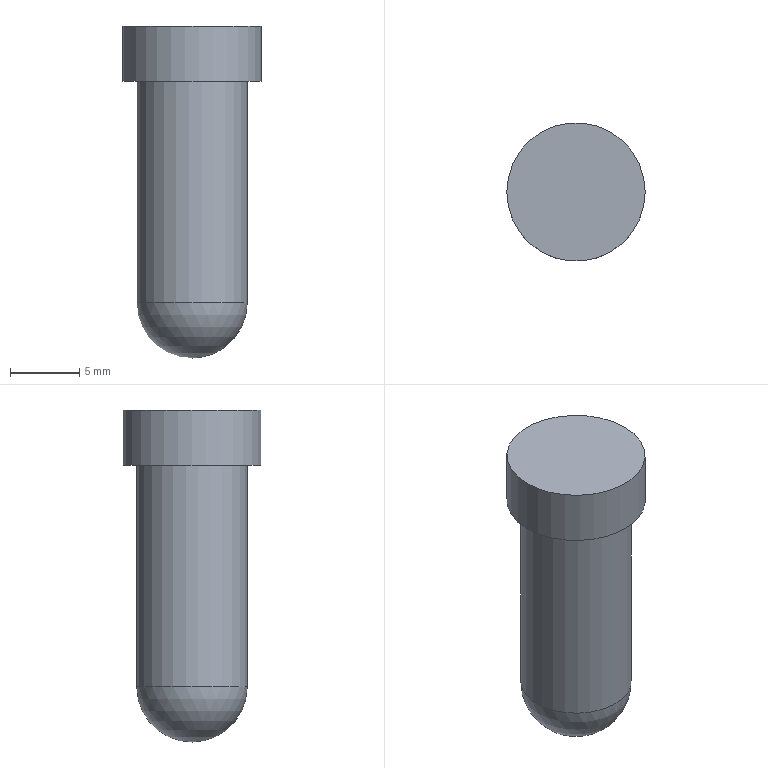Part | NX | features solid 2 | 1 solid | 5 faces | box 10 x 10 x 24 mm | volume 1252 mm3 | cylinder 2 | plane 2 | sphere 1 | commonest cylinder face diameters 8 x1 10 x1
STEP:
#1=CARTESIAN_POINT('',(-41.,110.,-78.));
#2=VERTEX_POINT('',#1);
#3=CARTESIAN_POINT('',(-45.,110.,-78.));
#4=DIRECTION('',(0.,0.,1.));
#5=DIRECTION('',(1.,0.,0.));
#6=AXIS2_PLACEMENT_3D('',#3,#4,#5);
#7=CIRCLE('',#6,4.);
#8=EDGE_CURVE('',#2,#2,#7,.F.);
#9=ORIENTED_EDGE('',*,*,#8,.F.);
#10=EDGE_LOOP('',(#9));
#11=FACE_BOUND('',#10,.T.);
#12=CARTESIAN_POINT('',(-41.,110.,-62.));
#13=VERTEX_POINT('',#12);
#14=CARTESIAN_POINT('',(-45.,110.,-62.));
#15=DIRECTION('',(0.,0.,1.));
#16=DIRECTION('',(1.,0.,0.));
#17=AXIS2_PLACEMENT_3D('',#14,#15,#16);
#18=CIRCLE('',#17,4.);
#19=EDGE_CURVE('',#13,#13,#18,.F.);
#20=ORIENTED_EDGE('',*,*,#19,.T.);
#21=EDGE_LOOP('',(#20));
#22=FACE_BOUND('',#21,.T.);
#23=CARTESIAN_POINT('',(-45.,110.,-62.));
#24=DIRECTION('',(0.,0.,-1.));
#25=DIRECTION('',(1.,0.,0.));
#26=AXIS2_PLACEMENT_3D('',#23,#24,#25);
#27=CYLINDRICAL_SURFACE('',#26,4.);
#28=ADVANCED_FACE('',(#11,#22),#27,.T.);
#29=ORIENTED_EDGE('',*,*,#8,.T.);
#30=EDGE_LOOP('',(#29));
#31=FACE_BOUND('',#30,.T.);
#32=CARTESIAN_POINT('',(-45.,110.,-78.));
#33=DIRECTION('',(0.,0.,-1.));
#34=DIRECTION('',(1.,0.,0.));
#35=AXIS2_PLACEMENT_3D('',#32,#33,#34);
#36=SPHERICAL_SURFACE('',#35,4.);
#37=ADVANCED_FACE('',(#31),#36,.T.);
#38=CARTESIAN_POINT('',(-40.,110.,-58.));
#39=VERTEX_POINT('',#38);
#40=CARTESIAN_POINT('',(-45.,110.,-58.));
#41=DIRECTION('',(0.,0.,1.));
#42=DIRECTION('',(1.,0.,0.));
#43=AXIS2_PLACEMENT_3D('',#40,#41,#42);
#44=CIRCLE('',#43,5.);
#45=EDGE_CURVE('',#39,#39,#44,.T.);
#46=ORIENTED_EDGE('',*,*,#45,.F.);
#47=EDGE_LOOP('',(#46));
#48=FACE_BOUND('',#47,.T.);
#49=CARTESIAN_POINT('',(-40.,110.,-62.));
#50=VERTEX_POINT('',#49);
#51=CARTESIAN_POINT('',(-45.,110.,-62.));
#52=DIRECTION('',(0.,0.,1.));
#53=DIRECTION('',(1.,0.,0.));
#54=AXIS2_PLACEMENT_3D('',#51,#52,#53);
#55=CIRCLE('',#54,5.);
#56=EDGE_CURVE('',#50,#50,#55,.T.);
#57=ORIENTED_EDGE('',*,*,#56,.T.);
#58=EDGE_LOOP('',(#57));
#59=FACE_BOUND('',#58,.T.);
#60=CARTESIAN_POINT('',(-45.,110.,-58.));
#61=DIRECTION('',(0.,0.,-1.));
#62=DIRECTION('',(1.,0.,0.));
#63=AXIS2_PLACEMENT_3D('',#60,#61,#62);
#64=CYLINDRICAL_SURFACE('',#63,5.);
#65=ADVANCED_FACE('',(#48,#59),#64,.T.);
#66=ORIENTED_EDGE('',*,*,#45,.T.);
#67=EDGE_LOOP('',(#66));
#68=FACE_BOUND('',#67,.T.);
#69=CARTESIAN_POINT('',(-45.,110.,-58.));
#70=DIRECTION('',(0.,0.,-1.));
#71=DIRECTION('',(1.,0.,0.));
#72=AXIS2_PLACEMENT_3D('',#69,#70,#71);
#73=PLANE('',#72);
#74=ADVANCED_FACE('',(#68),#73,.F.);
#75=ORIENTED_EDGE('',*,*,#19,.F.);
#76=EDGE_LOOP('',(#75));
#77=FACE_BOUND('',#76,.T.);
#78=ORIENTED_EDGE('',*,*,#56,.F.);
#79=EDGE_LOOP('',(#78));
#80=FACE_BOUND('',#79,.T.);
#81=CARTESIAN_POINT('',(-45.,110.,-62.));
#82=DIRECTION('',(0.,0.,-1.));
#83=DIRECTION('',(1.,0.,0.));
#84=AXIS2_PLACEMENT_3D('',#81,#82,#83);
#85=PLANE('',#84);
#86=ADVANCED_FACE('',(#77,#80),#85,.T.);
#87=CLOSED_SHELL('',(#28,#37,#65,#74,#86));
#88=MANIFOLD_SOLID_BREP('',#87);
#89=(LENGTH_UNIT()NAMED_UNIT(*)SI_UNIT(.MILLI.,.METRE.));
#90=UNCERTAINTY_MEASURE_WITH_UNIT(LENGTH_MEASURE(0.00001),#89,'','');
#91=(NAMED_UNIT(*)PLANE_ANGLE_UNIT()SI_UNIT($,.RADIAN.));
#92=(NAMED_UNIT(*)SI_UNIT($,.STERADIAN.)SOLID_ANGLE_UNIT());
#93=(GEOMETRIC_REPRESENTATION_CONTEXT(3)GLOBAL_UNCERTAINTY_ASSIGNED_CONTEXT((#90))GLOBAL_UNIT_ASSIGNED_CONTEXT((#89,#91,#92))REPRESENTATION_CONTEXT('',''));
#94=ADVANCED_BREP_SHAPE_REPRESENTATION('',(#88),#93);